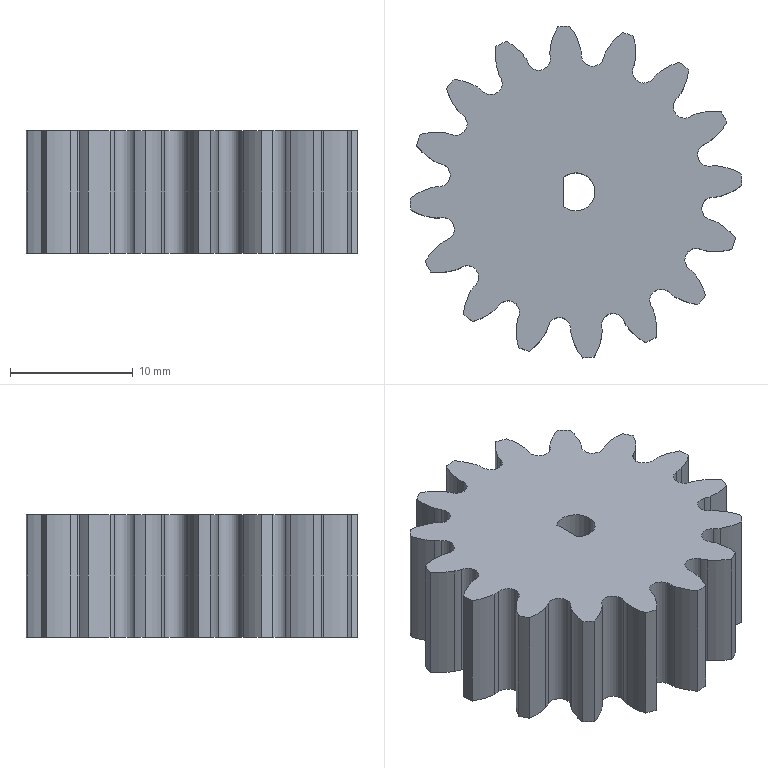Part | NX | features BREP 1, DATUM_CSYS 1 | 1 solid | 100 faces | box 26.979 x 26.979 x 10 mm | volume 4412 mm3 | cylinder 97 | plane 3 | commonest cylinder face diameters 4 x32 10.125 x32 1.86 x16 27 x16 3.1 x1